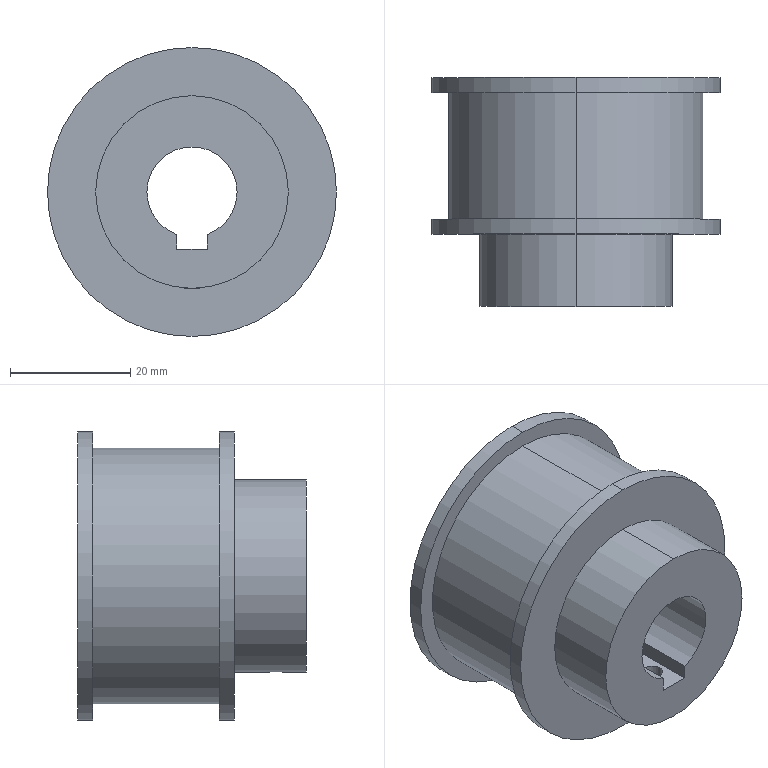Part | STEP file | PN_0055 (ATP14L075)_ATP22XL050-A-H8 | 1 solid | 19 faces | box 48 x 38 x 48 mm | volume 41242 mm3 | cylinder 11 | plane 8 | commonest cylinder face diameters 48 x4 3.3 x2 32 x2 42.45 x2 15 x1